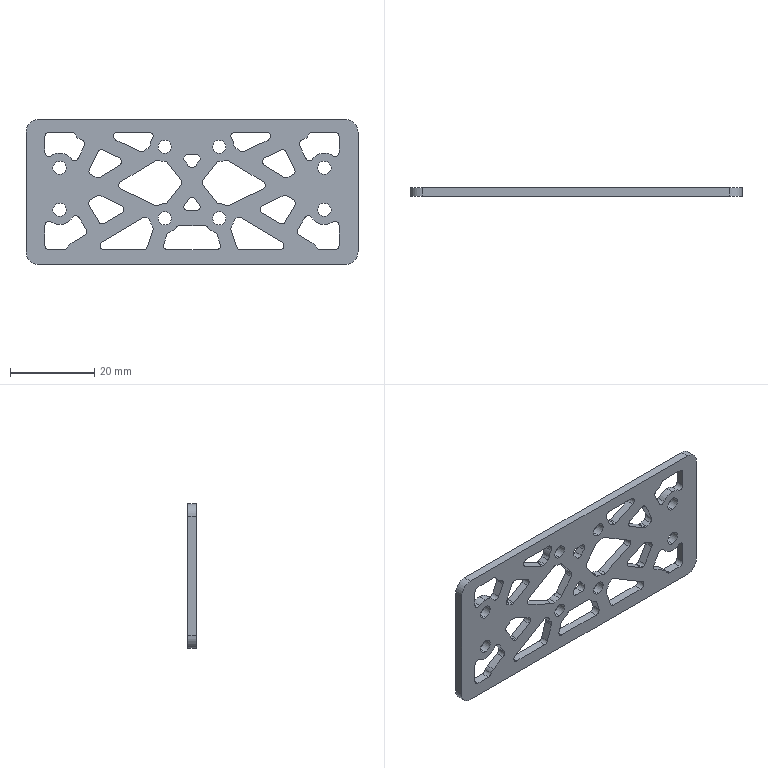Part | SolidWorks | features Fillet 2, Extrusion 1, ICE 1 | 1 solid | 201 faces | box 79 x 2 x 34.5 mm | volume 3709 mm3 | cylinder 131 | plane 70 | commonest cylinder face diameters 2 x91 3.2 x16 7 x16 3.5 x4 6 x4